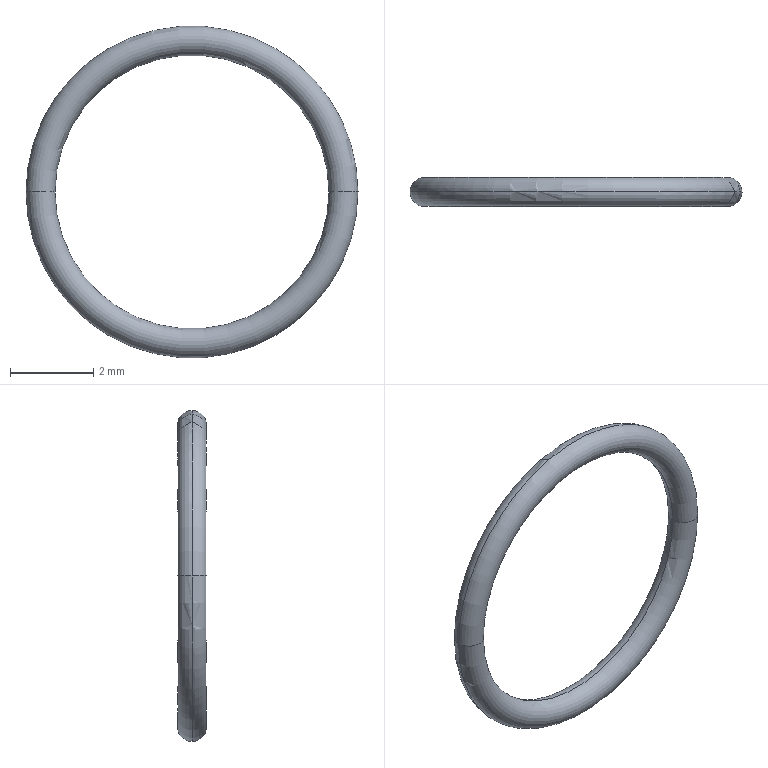Part | Creo | 1 solid | 4 faces | box 8 x 0.7 x 8 mm | volume 8.826 mm3 | torus 4
STEP:
#1=CARTESIAN_POINT('',(0.,0.,0.));
#2=DIRECTION('',(0.,0.,1.));
#3=DIRECTION('',(1.,0.,0.));
#4=AXIS2_PLACEMENT_3D('',#1,#2,#3);
#5=CARTESIAN_POINT('',(51.7,50.5,60.91));
#6=VERTEX_POINT('',#5);
#7=CARTESIAN_POINT('',(58.3,50.5,60.91));
#8=VERTEX_POINT('',#7);
#9=CARTESIAN_POINT('',(55.,50.5,60.91));
#10=DIRECTION('',(0.,1.,0.));
#11=DIRECTION('',(-1.,0.,0.));
#12=AXIS2_PLACEMENT_3D('',#9,#10,#11);
#13=CIRCLE('',#12,3.3);
#14=EDGE_CURVE('',#6,#8,#13,.T.);
#15=ORIENTED_EDGE('',*,*,#14,.F.);
#16=CARTESIAN_POINT('',(51.,50.5,60.91));
#17=VERTEX_POINT('',#16);
#18=CARTESIAN_POINT('',(51.35,50.5,60.91));
#19=DIRECTION('',(0.,0.,-1.));
#20=DIRECTION('',(1.,0.,0.));
#21=AXIS2_PLACEMENT_3D('',#18,#19,#20);
#22=CIRCLE('',#21,0.35);
#23=EDGE_CURVE('',#6,#17,#22,.T.);
#24=ORIENTED_EDGE('',*,*,#23,.T.);
#25=CARTESIAN_POINT('',(59.,50.5,60.91));
#26=VERTEX_POINT('',#25);
#27=CARTESIAN_POINT('',(55.,50.5,60.91));
#28=DIRECTION('',(0.,1.,0.));
#29=DIRECTION('',(-1.,0.,0.));
#30=AXIS2_PLACEMENT_3D('',#27,#28,#29);
#31=CIRCLE('',#30,4.);
#32=EDGE_CURVE('',#17,#26,#31,.T.);
#33=ORIENTED_EDGE('',*,*,#32,.T.);
#34=CARTESIAN_POINT('',(58.65,50.5,60.91));
#35=DIRECTION('',(0.,0.,1.));
#36=DIRECTION('',(-1.,0.,0.));
#37=AXIS2_PLACEMENT_3D('',#34,#35,#36);
#38=CIRCLE('',#37,0.35);
#39=EDGE_CURVE('',#8,#26,#38,.T.);
#40=ORIENTED_EDGE('',*,*,#39,.F.);
#41=EDGE_LOOP('',(#15,#24,#33,#40));
#42=FACE_OUTER_BOUND('',#41,.F.);
#43=CARTESIAN_POINT('',(55.,50.5,60.91));
#44=DIRECTION('',(0.,1.,0.));
#45=DIRECTION('',(-1.,0.,0.));
#46=AXIS2_PLACEMENT_3D('',#43,#44,#45);
#47=TOROIDAL_SURFACE('',#46,3.65,0.35);
#48=ADVANCED_FACE('',(#42),#47,.T.);
#49=ORIENTED_EDGE('',*,*,#32,.F.);
#50=CARTESIAN_POINT('',(51.35,50.5,60.91));
#51=DIRECTION('',(0.,0.,-1.));
#52=DIRECTION('',(-1.,0.,0.));
#53=AXIS2_PLACEMENT_3D('',#50,#51,#52);
#54=CIRCLE('',#53,0.35);
#55=EDGE_CURVE('',#17,#6,#54,.T.);
#56=ORIENTED_EDGE('',*,*,#55,.T.);
#57=ORIENTED_EDGE('',*,*,#14,.T.);
#58=CARTESIAN_POINT('',(58.65,50.5,60.91));
#59=DIRECTION('',(0.,0.,1.));
#60=DIRECTION('',(1.,0.,0.));
#61=AXIS2_PLACEMENT_3D('',#58,#59,#60);
#62=CIRCLE('',#61,0.35);
#63=EDGE_CURVE('',#26,#8,#62,.T.);
#64=ORIENTED_EDGE('',*,*,#63,.F.);
#65=EDGE_LOOP('',(#49,#56,#57,#64));
#66=FACE_OUTER_BOUND('',#65,.F.);
#67=CARTESIAN_POINT('',(55.,50.5,60.91));
#68=DIRECTION('',(0.,1.,0.));
#69=DIRECTION('',(-1.,0.,0.));
#70=AXIS2_PLACEMENT_3D('',#67,#68,#69);
#71=TOROIDAL_SURFACE('',#70,3.65,0.35);
#72=ADVANCED_FACE('',(#66),#71,.T.);
#73=CARTESIAN_POINT('',(55.,50.5,60.91));
#74=DIRECTION('',(0.,1.,0.));
#75=DIRECTION('',(1.,0.,0.));
#76=AXIS2_PLACEMENT_3D('',#73,#74,#75);
#77=CIRCLE('',#76,4.);
#78=EDGE_CURVE('',#26,#17,#77,.T.);
#79=ORIENTED_EDGE('',*,*,#78,.F.);
#80=ORIENTED_EDGE('',*,*,#63,.T.);
#81=CARTESIAN_POINT('',(55.,50.5,60.91));
#82=DIRECTION('',(0.,1.,0.));
#83=DIRECTION('',(1.,0.,0.));
#84=AXIS2_PLACEMENT_3D('',#81,#82,#83);
#85=CIRCLE('',#84,3.3);
#86=EDGE_CURVE('',#8,#6,#85,.T.);
#87=ORIENTED_EDGE('',*,*,#86,.T.);
#88=ORIENTED_EDGE('',*,*,#55,.F.);
#89=EDGE_LOOP('',(#79,#80,#87,#88));
#90=FACE_OUTER_BOUND('',#89,.F.);
#91=CARTESIAN_POINT('',(55.,50.5,60.91));
#92=DIRECTION('',(0.,1.,0.));
#93=DIRECTION('',(-1.,0.,0.));
#94=AXIS2_PLACEMENT_3D('',#91,#92,#93);
#95=TOROIDAL_SURFACE('',#94,3.65,0.35);
#96=ADVANCED_FACE('',(#90),#95,.T.);
#97=ORIENTED_EDGE('',*,*,#86,.F.);
#98=ORIENTED_EDGE('',*,*,#39,.T.);
#99=ORIENTED_EDGE('',*,*,#78,.T.);
#100=ORIENTED_EDGE('',*,*,#23,.F.);
#101=EDGE_LOOP('',(#97,#98,#99,#100));
#102=FACE_OUTER_BOUND('',#101,.F.);
#103=CARTESIAN_POINT('',(55.,50.5,60.91));
#104=DIRECTION('',(0.,1.,0.));
#105=DIRECTION('',(-1.,0.,0.));
#106=AXIS2_PLACEMENT_3D('',#103,#104,#105);
#107=TOROIDAL_SURFACE('',#106,3.65,0.35);
#108=ADVANCED_FACE('',(#102),#107,.T.);
#109=CLOSED_SHELL('',(#48,#72,#96,#108));
#110=MANIFOLD_SOLID_BREP('',#109);
#111=(LENGTH_UNIT()NAMED_UNIT(*)SI_UNIT(.MILLI.,.METRE.));
#112=UNCERTAINTY_MEASURE_WITH_UNIT(LENGTH_MEASURE(0.001133),#111,'','');
#113=(NAMED_UNIT(*)PLANE_ANGLE_UNIT()SI_UNIT($,.RADIAN.));
#114=PLANE_ANGLE_MEASURE_WITH_UNIT(PLANE_ANGLE_MEASURE(0.01745),#113);
#115=(CONVERSION_BASED_UNIT('DEGREE',#114)NAMED_UNIT(*)PLANE_ANGLE_UNIT());
#116=(NAMED_UNIT(*)SI_UNIT($,.STERADIAN.)SOLID_ANGLE_UNIT());
#117=(GEOMETRIC_REPRESENTATION_CONTEXT(3)GLOBAL_UNCERTAINTY_ASSIGNED_CONTEXT((#112))GLOBAL_UNIT_ASSIGNED_CONTEXT((#111,#115,#116))REPRESENTATION_CONTEXT('',''));
#118=ADVANCED_BREP_SHAPE_REPRESENTATION('',(#4,#110),#117);